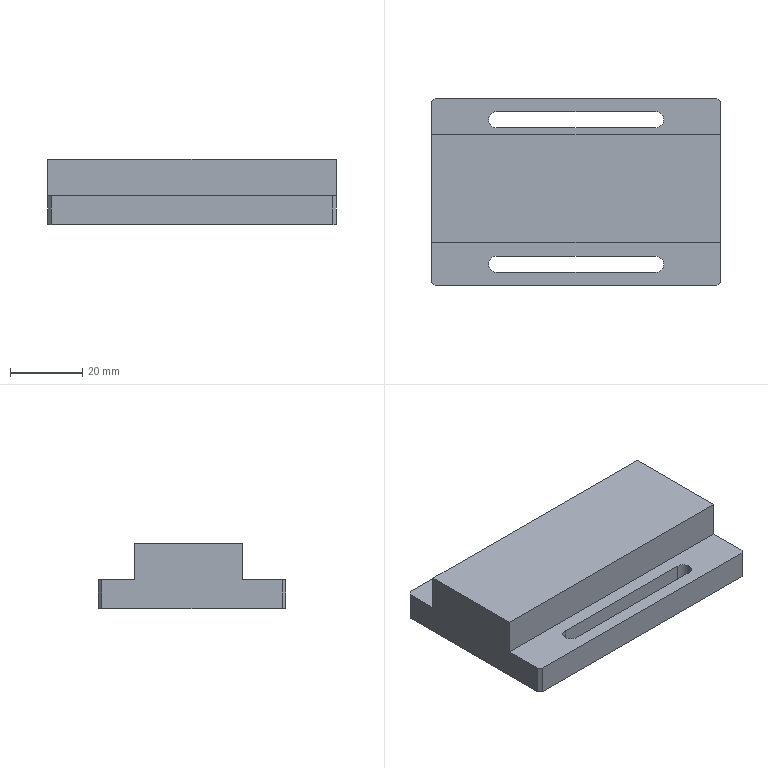Part | STEP file | ASND-0110-Body 1-21 | 1 solid | 24 faces | box 80 x 52 x 18 mm | volume 53842 mm3 | plane 18 | cylinder 6 | commonest cylinder face diameters 4.5 x6